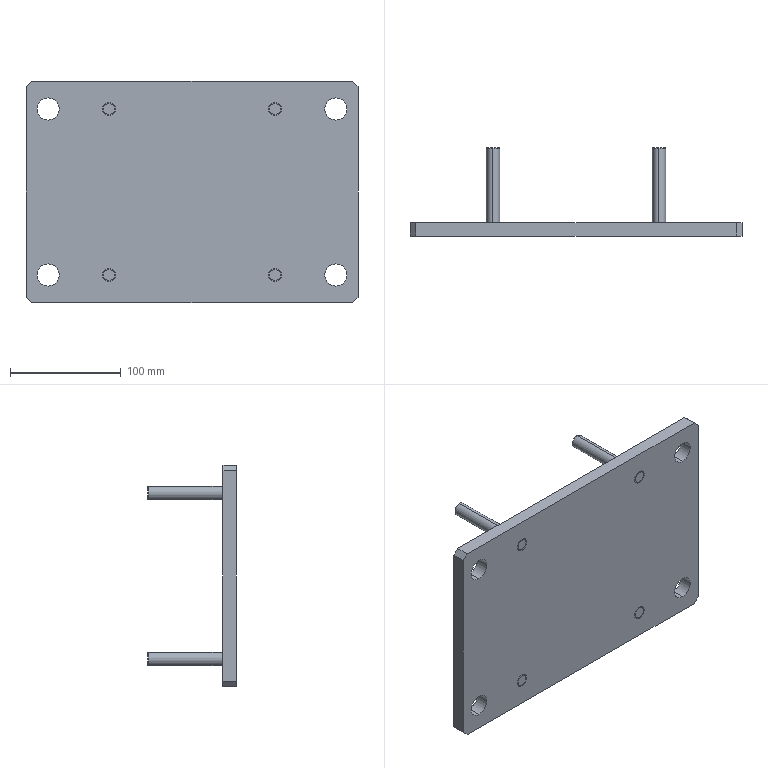Part | SolidWorks | features Chamfer 2, HoleWzd 2, Extrusion 1, ICE 1, SketchPattern 1 | 6 solids | 56 faces | box 300 x 80 x 200 mm | volume 745614 mm3 | cylinder 26 | plane 20 | cone 10 | commonest cylinder face diameters 12 x10 10.2 x8 20 x8
STEP:
#1=CARTESIAN_POINT('',(75.,74.,80.5));
#2=VERTEX_POINT('',#1);
#3=CARTESIAN_POINT('',(75.,74.,69.5));
#4=VERTEX_POINT('',#3);
#5=CARTESIAN_POINT('',(75.,74.,75.));
#6=DIRECTION('',(0.,1.,0.));
#7=DIRECTION('',(0.,0.,-1.));
#8=AXIS2_PLACEMENT_3D('',#5,#6,#7);
#9=CIRCLE('',#8,5.5);
#10=EDGE_CURVE('',#2,#4,#9,.T.);
#11=ORIENTED_EDGE('',*,*,#10,.F.);
#12=CARTESIAN_POINT('',(75.,73.5,81.));
#13=VERTEX_POINT('',#12);
#14=CARTESIAN_POINT('',(75.,73.5,81.));
#15=DIRECTION('',(0.,-0.7071,0.7071));
#16=VECTOR('',#15,1000.);
#17=LINE('',#14,#16);
#18=EDGE_CURVE('',#2,#13,#17,.T.);
#19=ORIENTED_EDGE('',*,*,#18,.T.);
#20=CARTESIAN_POINT('',(75.,73.5,69.));
#21=VERTEX_POINT('',#20);
#22=CARTESIAN_POINT('',(75.,73.5,75.));
#23=DIRECTION('',(0.,-1.,0.));
#24=DIRECTION('',(0.,0.,-1.));
#25=AXIS2_PLACEMENT_3D('',#22,#23,#24);
#26=CIRCLE('',#25,6.);
#27=EDGE_CURVE('',#21,#13,#26,.T.);
#28=ORIENTED_EDGE('',*,*,#27,.F.);
#29=CARTESIAN_POINT('',(75.,73.5,69.));
#30=DIRECTION('',(0.,-0.7071,-0.7071));
#31=VECTOR('',#30,1000.);
#32=LINE('',#29,#31);
#33=EDGE_CURVE('',#4,#21,#32,.T.);
#34=ORIENTED_EDGE('',*,*,#33,.F.);
#35=EDGE_LOOP('',(#11,#19,#28,#34));
#36=FACE_OUTER_BOUND('',#35,.T.);
#37=CARTESIAN_POINT('',(75.,73.5,75.));
#38=DIRECTION('',(0.,-1.,0.));
#39=DIRECTION('',(0.,0.,-1.));
#40=AXIS2_PLACEMENT_3D('',#37,#38,#39);
#41=CONICAL_SURFACE('',#40,6.,0.7854);
#42=ADVANCED_FACE('',(#36),#41,.T.);
#43=ORIENTED_EDGE('',*,*,#27,.T.);
#44=CARTESIAN_POINT('',(75.,-6.,81.));
#45=VERTEX_POINT('',#44);
#46=CARTESIAN_POINT('',(75.,74.,81.));
#47=DIRECTION('',(0.,-1.,0.));
#48=VECTOR('',#47,1000.);
#49=LINE('',#46,#48);
#50=EDGE_CURVE('',#13,#45,#49,.T.);
#51=ORIENTED_EDGE('',*,*,#50,.T.);
#52=CARTESIAN_POINT('',(75.,-6.,69.));
#53=VERTEX_POINT('',#52);
#54=CARTESIAN_POINT('',(75.,-6.,75.));
#55=DIRECTION('',(0.,-1.,0.));
#56=DIRECTION('',(0.,0.,-1.));
#57=AXIS2_PLACEMENT_3D('',#54,#55,#56);
#58=CIRCLE('',#57,6.);
#59=EDGE_CURVE('',#53,#45,#58,.T.);
#60=ORIENTED_EDGE('',*,*,#59,.F.);
#61=CARTESIAN_POINT('',(75.,74.,69.));
#62=DIRECTION('',(0.,-1.,0.));
#63=VECTOR('',#62,1000.);
#64=LINE('',#61,#63);
#65=EDGE_CURVE('',#21,#53,#64,.T.);
#66=ORIENTED_EDGE('',*,*,#65,.F.);
#67=EDGE_LOOP('',(#43,#51,#60,#66));
#68=FACE_OUTER_BOUND('',#67,.T.);
#69=CARTESIAN_POINT('',(75.,74.,75.));
#70=DIRECTION('',(0.,-1.,0.));
#71=DIRECTION('',(0.,0.,-1.));
#72=AXIS2_PLACEMENT_3D('',#69,#70,#71);
#73=CYLINDRICAL_SURFACE('',#72,6.);
#74=ADVANCED_FACE('',(#68),#73,.T.);
#75=ORIENTED_EDGE('',*,*,#50,.F.);
#76=CARTESIAN_POINT('',(75.,73.5,75.));
#77=DIRECTION('',(0.,-1.,0.));
#78=DIRECTION('',(0.,0.,-1.));
#79=AXIS2_PLACEMENT_3D('',#76,#77,#78);
#80=CIRCLE('',#79,6.);
#81=EDGE_CURVE('',#13,#21,#80,.T.);
#82=ORIENTED_EDGE('',*,*,#81,.T.);
#83=ORIENTED_EDGE('',*,*,#65,.T.);
#84=CARTESIAN_POINT('',(75.,-6.,75.));
#85=DIRECTION('',(0.,-1.,0.));
#86=DIRECTION('',(0.,0.,-1.));
#87=AXIS2_PLACEMENT_3D('',#84,#85,#86);
#88=CIRCLE('',#87,6.);
#89=EDGE_CURVE('',#45,#53,#88,.T.);
#90=ORIENTED_EDGE('',*,*,#89,.F.);
#91=EDGE_LOOP('',(#75,#82,#83,#90));
#92=FACE_OUTER_BOUND('',#91,.T.);
#93=CARTESIAN_POINT('',(75.,74.,75.));
#94=DIRECTION('',(0.,-1.,0.));
#95=DIRECTION('',(0.,0.,-1.));
#96=AXIS2_PLACEMENT_3D('',#93,#94,#95);
#97=CYLINDRICAL_SURFACE('',#96,6.);
#98=ADVANCED_FACE('',(#92),#97,.T.);
#99=CARTESIAN_POINT('',(75.,74.,75.));
#100=DIRECTION('',(0.,1.,0.));
#101=DIRECTION('',(0.,0.,-1.));
#102=AXIS2_PLACEMENT_3D('',#99,#100,#101);
#103=CIRCLE('',#102,5.5);
#104=EDGE_CURVE('',#4,#2,#103,.T.);
#105=ORIENTED_EDGE('',*,*,#104,.T.);
#106=ORIENTED_EDGE('',*,*,#10,.T.);
#107=EDGE_LOOP('',(#105,#106));
#108=FACE_OUTER_BOUND('',#107,.T.);
#109=CARTESIAN_POINT('',(75.,74.,75.));
#110=DIRECTION('',(0.,-1.,0.));
#111=DIRECTION('',(0.,0.,-1.));
#112=AXIS2_PLACEMENT_3D('',#109,#110,#111);
#113=PLANE('',#112);
#114=ADVANCED_FACE('',(#108),#113,.F.);
#115=ORIENTED_EDGE('',*,*,#59,.T.);
#116=ORIENTED_EDGE('',*,*,#89,.T.);
#117=EDGE_LOOP('',(#115,#116));
#118=FACE_OUTER_BOUND('',#117,.T.);
#119=CARTESIAN_POINT('',(75.,-6.,75.));
#120=DIRECTION('',(0.,-1.,0.));
#121=DIRECTION('',(0.,0.,-1.));
#122=AXIS2_PLACEMENT_3D('',#119,#120,#121);
#123=PLANE('',#122);
#124=ADVANCED_FACE('',(#118),#123,.T.);
#125=ORIENTED_EDGE('',*,*,#18,.F.);
#126=ORIENTED_EDGE('',*,*,#104,.F.);
#127=ORIENTED_EDGE('',*,*,#33,.T.);
#128=ORIENTED_EDGE('',*,*,#81,.F.);
#129=EDGE_LOOP('',(#125,#126,#127,#128));
#130=FACE_OUTER_BOUND('',#129,.T.);
#131=CARTESIAN_POINT('',(75.,73.5,75.));
#132=DIRECTION('',(0.,-1.,0.));
#133=DIRECTION('',(0.,0.,-1.));
#134=AXIS2_PLACEMENT_3D('',#131,#132,#133);
#135=CONICAL_SURFACE('',#134,6.,0.7854);
#136=ADVANCED_FACE('',(#130),#135,.T.);
#137=CLOSED_SHELL('',(#42,#74,#98,#114,#124,#136));
#138=MANIFOLD_SOLID_BREP('',#137);
#139=CARTESIAN_POINT('',(75.,74.,80.5));
#140=VERTEX_POINT('',#139);
#141=CARTESIAN_POINT('',(75.,74.,69.5));
#142=VERTEX_POINT('',#141);
#143=CARTESIAN_POINT('',(75.,74.,75.));
#144=DIRECTION('',(0.,1.,0.));
#145=DIRECTION('',(0.,0.,-1.));
#146=AXIS2_PLACEMENT_3D('',#143,#144,#145);
#147=CIRCLE('',#146,5.5);
#148=EDGE_CURVE('',#140,#142,#147,.T.);
#149=ORIENTED_EDGE('',*,*,#148,.F.);
#150=CARTESIAN_POINT('',(75.,73.5,81.));
#151=VERTEX_POINT('',#150);
#152=CARTESIAN_POINT('',(75.,73.5,81.));
#153=DIRECTION('',(0.,-0.7071,0.7071));
#154=VECTOR('',#153,1000.);
#155=LINE('',#152,#154);
#156=EDGE_CURVE('',#140,#151,#155,.T.);
#157=ORIENTED_EDGE('',*,*,#156,.T.);
#158=CARTESIAN_POINT('',(75.,73.5,69.));
#159=VERTEX_POINT('',#158);
#160=CARTESIAN_POINT('',(75.,73.5,75.));
#161=DIRECTION('',(0.,-1.,0.));
#162=DIRECTION('',(0.,0.,-1.));
#163=AXIS2_PLACEMENT_3D('',#160,#161,#162);
#164=CIRCLE('',#163,6.);
#165=EDGE_CURVE('',#159,#151,#164,.T.);
#166=ORIENTED_EDGE('',*,*,#165,.F.);
#167=CARTESIAN_POINT('',(75.,73.5,69.));
#168=DIRECTION('',(0.,-0.7071,-0.7071));
#169=VECTOR('',#168,1000.);
#170=LINE('',#167,#169);
#171=EDGE_CURVE('',#142,#159,#170,.T.);
#172=ORIENTED_EDGE('',*,*,#171,.F.);
#173=EDGE_LOOP('',(#149,#157,#166,#172));
#174=FACE_OUTER_BOUND('',#173,.T.);
#175=CARTESIAN_POINT('',(75.,73.5,75.));
#176=DIRECTION('',(0.,-1.,0.));
#177=DIRECTION('',(0.,0.,-1.));
#178=AXIS2_PLACEMENT_3D('',#175,#176,#177);
#179=CONICAL_SURFACE('',#178,6.,0.7854);
#180=ADVANCED_FACE('',(#174),#179,.T.);
#181=ORIENTED_EDGE('',*,*,#165,.T.);
#182=CARTESIAN_POINT('',(75.,-6.,81.));
#183=VERTEX_POINT('',#182);
#184=CARTESIAN_POINT('',(75.,74.,81.));
#185=DIRECTION('',(0.,-1.,0.));
#186=VECTOR('',#185,1000.);
#187=LINE('',#184,#186);
#188=EDGE_CURVE('',#151,#183,#187,.T.);
#189=ORIENTED_EDGE('',*,*,#188,.T.);
#190=CARTESIAN_POINT('',(75.,-6.,69.));
#191=VERTEX_POINT('',#190);
#192=CARTESIAN_POINT('',(75.,-6.,75.));
#193=DIRECTION('',(0.,-1.,0.));
#194=DIRECTION('',(0.,0.,-1.));
#195=AXIS2_PLACEMENT_3D('',#192,#193,#194);
#196=CIRCLE('',#195,6.);
#197=EDGE_CURVE('',#191,#183,#196,.T.);
#198=ORIENTED_EDGE('',*,*,#197,.F.);
#199=CARTESIAN_POINT('',(75.,74.,69.));
#200=DIRECTION('',(0.,-1.,0.));
#201=VECTOR('',#200,1000.);
#202=LINE('',#199,#201);
#203=EDGE_CURVE('',#159,#191,#202,.T.);
#204=ORIENTED_EDGE('',*,*,#203,.F.);
#205=EDGE_LOOP('',(#181,#189,#198,#204));
#206=FACE_OUTER_BOUND('',#205,.T.);
#207=CARTESIAN_POINT('',(75.,74.,75.));
#208=DIRECTION('',(0.,-1.,0.));
#209=DIRECTION('',(0.,0.,-1.));
#210=AXIS2_PLACEMENT_3D('',#207,#208,#209);
#211=CYLINDRICAL_SURFACE('',#210,6.);
#212=ADVANCED_FACE('',(#206),#211,.T.);
#213=ORIENTED_EDGE('',*,*,#188,.F.);
#214=CARTESIAN_POINT('',(75.,73.5,75.));
#215=DIRECTION('',(0.,-1.,0.));
#216=DIRECTION('',(0.,0.,-1.));
#217=AXIS2_PLACEMENT_3D('',#214,#215,#216);
#218=CIRCLE('',#217,6.);
#219=EDGE_CURVE('',#151,#159,#218,.T.);
#220=ORIENTED_EDGE('',*,*,#219,.T.);
#221=ORIENTED_EDGE('',*,*,#203,.T.);
#222=CARTESIAN_POINT('',(75.,-6.,75.));
#223=DIRECTION('',(0.,-1.,0.));
#224=DIRECTION('',(0.,0.,-1.));
#225=AXIS2_PLACEMENT_3D('',#222,#223,#224);
#226=CIRCLE('',#225,6.);
#227=EDGE_CURVE('',#183,#191,#226,.T.);
#228=ORIENTED_EDGE('',*,*,#227,.F.);
#229=EDGE_LOOP('',(#213,#220,#221,#228));
#230=FACE_OUTER_BOUND('',#229,.T.);
#231=CARTESIAN_POINT('',(75.,74.,75.));
#232=DIRECTION('',(0.,-1.,0.));
#233=DIRECTION('',(0.,0.,-1.));
#234=AXIS2_PLACEMENT_3D('',#231,#232,#233);
#235=CYLINDRICAL_SURFACE('',#234,6.);
#236=ADVANCED_FACE('',(#230),#235,.T.);
#237=CARTESIAN_POINT('',(75.,74.,75.));
#238=DIRECTION('',(0.,1.,0.));
#239=DIRECTION('',(0.,0.,-1.));
#240=AXIS2_PLACEMENT_3D('',#237,#238,#239);
#241=CIRCLE('',#240,5.5);
#242=EDGE_CURVE('',#142,#140,#241,.T.);
#243=ORIENTED_EDGE('',*,*,#242,.T.);
#244=ORIENTED_EDGE('',*,*,#148,.T.);
#245=EDGE_LOOP('',(#243,#244));
#246=FACE_OUTER_BOUND('',#245,.T.);
#247=CARTESIAN_POINT('',(75.,74.,75.));
#248=DIRECTION('',(0.,-1.,0.));
#249=DIRECTION('',(0.,0.,-1.));
#250=AXIS2_PLACEMENT_3D('',#247,#248,#249);
#251=PLANE('',#250);
#252=ADVANCED_FACE('',(#246),#251,.F.);
#253=ORIENTED_EDGE('',*,*,#197,.T.);
#254=ORIENTED_EDGE('',*,*,#227,.T.);
#255=EDGE_LOOP('',(#253,#254));
#256=FACE_OUTER_BOUND('',#255,.T.);
#257=CARTESIAN_POINT('',(75.,-6.,75.));
#258=DIRECTION('',(0.,-1.,0.));
#259=DIRECTION('',(0.,0.,-1.));
#260=AXIS2_PLACEMENT_3D('',#257,#258,#259);
#261=PLANE('',#260);
#262=ADVANCED_FACE('',(#256),#261,.T.);
#263=ORIENTED_EDGE('',*,*,#156,.F.);
#264=ORIENTED_EDGE('',*,*,#242,.F.);
#265=ORIENTED_EDGE('',*,*,#171,.T.);
#266=ORIENTED_EDGE('',*,*,#219,.F.);
#267=EDGE_LOOP('',(#263,#264,#265,#266));
#268=FACE_OUTER_BOUND('',#267,.T.);
#269=CARTESIAN_POINT('',(75.,73.5,75.));
#270=DIRECTION('',(0.,-1.,0.));
#271=DIRECTION('',(0.,0.,-1.));
#272=AXIS2_PLACEMENT_3D('',#269,#270,#271);
#273=CONICAL_SURFACE('',#272,6.,0.7854);
#274=ADVANCED_FACE('',(#268),#273,.T.);
#275=CLOSED_SHELL('',(#180,#212,#236,#252,#262,#274));
#276=MANIFOLD_SOLID_BREP('',#275);
#277=CARTESIAN_POINT('',(75.,74.,-69.5));
#278=VERTEX_POINT('',#277);
#279=CARTESIAN_POINT('',(75.,74.,-80.5));
#280=VERTEX_POINT('',#279);
#281=CARTESIAN_POINT('',(75.,74.,-75.));
#282=DIRECTION('',(0.,1.,0.));
#283=DIRECTION('',(0.,0.,-1.));
#284=AXIS2_PLACEMENT_3D('',#281,#282,#283);
#285=CIRCLE('',#284,5.5);
#286=EDGE_CURVE('',#278,#280,#285,.T.);
#287=ORIENTED_EDGE('',*,*,#286,.F.);
#288=CARTESIAN_POINT('',(75.,73.5,-69.));
#289=VERTEX_POINT('',#288);
#290=CARTESIAN_POINT('',(75.,73.5,-69.));
#291=DIRECTION('',(0.,-0.7071,0.7071));
#292=VECTOR('',#291,1000.);
#293=LINE('',#290,#292);
#294=EDGE_CURVE('',#278,#289,#293,.T.);
#295=ORIENTED_EDGE('',*,*,#294,.T.);
#296=CARTESIAN_POINT('',(75.,73.5,-81.));
#297=VERTEX_POINT('',#296);
#298=CARTESIAN_POINT('',(75.,73.5,-75.));
#299=DIRECTION('',(0.,-1.,0.));
#300=DIRECTION('',(0.,0.,-1.));
#301=AXIS2_PLACEMENT_3D('',#298,#299,#300);
#302=CIRCLE('',#301,6.);
#303=EDGE_CURVE('',#297,#289,#302,.T.);
#304=ORIENTED_EDGE('',*,*,#303,.F.);
#305=CARTESIAN_POINT('',(75.,73.5,-81.));
#306=DIRECTION('',(0.,-0.7071,-0.7071));
#307=VECTOR('',#306,1000.);
#308=LINE('',#305,#307);
#309=EDGE_CURVE('',#280,#297,#308,.T.);
#310=ORIENTED_EDGE('',*,*,#309,.F.);
#311=EDGE_LOOP('',(#287,#295,#304,#310));
#312=FACE_OUTER_BOUND('',#311,.T.);
#313=CARTESIAN_POINT('',(75.,73.5,-75.));
#314=DIRECTION('',(0.,-1.,0.));
#315=DIRECTION('',(0.,0.,-1.));
#316=AXIS2_PLACEMENT_3D('',#313,#314,#315);
#317=CONICAL_SURFACE('',#316,6.,0.7854);
#318=ADVANCED_FACE('',(#312),#317,.T.);
#319=ORIENTED_EDGE('',*,*,#303,.T.);
#320=CARTESIAN_POINT('',(75.,-6.,-69.));
#321=VERTEX_POINT('',#320);
#322=CARTESIAN_POINT('',(75.,74.,-69.));
#323=DIRECTION('',(0.,-1.,0.));
#324=VECTOR('',#323,1000.);
#325=LINE('',#322,#324);
#326=EDGE_CURVE('',#289,#321,#325,.T.);
#327=ORIENTED_EDGE('',*,*,#326,.T.);
#328=CARTESIAN_POINT('',(75.,-6.,-81.));
#329=VERTEX_POINT('',#328);
#330=CARTESIAN_POINT('',(75.,-6.,-75.));
#331=DIRECTION('',(0.,-1.,0.));
#332=DIRECTION('',(0.,0.,-1.));
#333=AXIS2_PLACEMENT_3D('',#330,#331,#332);
#334=CIRCLE('',#333,6.);
#335=EDGE_CURVE('',#329,#321,#334,.T.);
#336=ORIENTED_EDGE('',*,*,#335,.F.);
#337=CARTESIAN_POINT('',(75.,74.,-81.));
#338=DIRECTION('',(0.,-1.,0.));
#339=VECTOR('',#338,1000.);
#340=LINE('',#337,#339);
#341=EDGE_CURVE('',#297,#329,#340,.T.);
#342=ORIENTED_EDGE('',*,*,#341,.F.);
#343=EDGE_LOOP('',(#319,#327,#336,#342));
#344=FACE_OUTER_BOUND('',#343,.T.);
#345=CARTESIAN_POINT('',(75.,74.,-75.));
#346=DIRECTION('',(0.,-1.,0.));
#347=DIRECTION('',(0.,0.,-1.));
#348=AXIS2_PLACEMENT_3D('',#345,#346,#347);
#349=CYLINDRICAL_SURFACE('',#348,6.);
#350=ADVANCED_FACE('',(#344),#349,.T.);
#351=ORIENTED_EDGE('',*,*,#326,.F.);
#352=CARTESIAN_POINT('',(75.,73.5,-75.));
#353=DIRECTION('',(0.,-1.,0.));
#354=DIRECTION('',(0.,0.,-1.));
#355=AXIS2_PLACEMENT_3D('',#352,#353,#354);
#356=CIRCLE('',#355,6.);
#357=EDGE_CURVE('',#289,#297,#356,.T.);
#358=ORIENTED_EDGE('',*,*,#357,.T.);
#359=ORIENTED_EDGE('',*,*,#341,.T.);
#360=CARTESIAN_POINT('',(75.,-6.,-75.));
#361=DIRECTION('',(0.,-1.,0.));
#362=DIRECTION('',(0.,0.,-1.));
#363=AXIS2_PLACEMENT_3D('',#360,#361,#362);
#364=CIRCLE('',#363,6.);
#365=EDGE_CURVE('',#321,#329,#364,.T.);
#366=ORIENTED_EDGE('',*,*,#365,.F.);
#367=EDGE_LOOP('',(#351,#358,#359,#366));
#368=FACE_OUTER_BOUND('',#367,.T.);
#369=CARTESIAN_POINT('',(75.,74.,-75.));
#370=DIRECTION('',(0.,-1.,0.));
#371=DIRECTION('',(0.,0.,-1.));
#372=AXIS2_PLACEMENT_3D('',#369,#370,#371);
#373=CYLINDRICAL_SURFACE('',#372,6.);
#374=ADVANCED_FACE('',(#368),#373,.T.);
#375=CARTESIAN_POINT('',(75.,74.,-75.));
#376=DIRECTION('',(0.,1.,0.));
#377=DIRECTION('',(0.,0.,-1.));
#378=AXIS2_PLACEMENT_3D('',#375,#376,#377);
#379=CIRCLE('',#378,5.5);
#380=EDGE_CURVE('',#280,#278,#379,.T.);
#381=ORIENTED_EDGE('',*,*,#380,.T.);
#382=ORIENTED_EDGE('',*,*,#286,.T.);
#383=EDGE_LOOP('',(#381,#382));
#384=FACE_OUTER_BOUND('',#383,.T.);
#385=CARTESIAN_POINT('',(75.,74.,-75.));
#386=DIRECTION('',(0.,-1.,0.));
#387=DIRECTION('',(0.,0.,-1.));
#388=AXIS2_PLACEMENT_3D('',#385,#386,#387);
#389=PLANE('',#388);
#390=ADVANCED_FACE('',(#384),#389,.F.);
#391=ORIENTED_EDGE('',*,*,#335,.T.);
#392=ORIENTED_EDGE('',*,*,#365,.T.);
#393=EDGE_LOOP('',(#391,#392));
#394=FACE_OUTER_BOUND('',#393,.T.);
#395=CARTESIAN_POINT('',(75.,-6.,-75.));
#396=DIRECTION('',(0.,-1.,0.));
#397=DIRECTION('',(0.,0.,-1.));
#398=AXIS2_PLACEMENT_3D('',#395,#396,#397);
#399=PLANE('',#398);
#400=ADVANCED_FACE('',(#394),#399,.T.);
#401=ORIENTED_EDGE('',*,*,#294,.F.);
#402=ORIENTED_EDGE('',*,*,#380,.F.);
#403=ORIENTED_EDGE('',*,*,#309,.T.);
#404=ORIENTED_EDGE('',*,*,#357,.F.);
#405=EDGE_LOOP('',(#401,#402,#403,#404));
#406=FACE_OUTER_BOUND('',#405,.T.);
#407=CARTESIAN_POINT('',(75.,73.5,-75.));
#408=DIRECTION('',(0.,-1.,0.));
#409=DIRECTION('',(0.,0.,-1.));
#410=AXIS2_PLACEMENT_3D('',#407,#408,#409);
#411=CONICAL_SURFACE('',#410,6.,0.7854);
#412=ADVANCED_FACE('',(#406),#411,.T.);
#413=CLOSED_SHELL('',(#318,#350,#374,#390,#400,#412));
#414=MANIFOLD_SOLID_BREP('',#413);
#415=CARTESIAN_POINT('',(-75.,74.,-69.5));
#416=VERTEX_POINT('',#415);
#417=CARTESIAN_POINT('',(-75.,74.,-80.5));
#418=VERTEX_POINT('',#417);
#419=CARTESIAN_POINT('',(-75.,74.,-75.));
#420=DIRECTION('',(0.,1.,0.));
#421=DIRECTION('',(0.,0.,-1.));
#422=AXIS2_PLACEMENT_3D('',#419,#420,#421);
#423=CIRCLE('',#422,5.5);
#424=EDGE_CURVE('',#416,#418,#423,.T.);
#425=ORIENTED_EDGE('',*,*,#424,.F.);
#426=CARTESIAN_POINT('',(-75.,73.5,-69.));
#427=VERTEX_POINT('',#426);
#428=CARTESIAN_POINT('',(-75.,73.5,-69.));
#429=DIRECTION('',(0.,-0.7071,0.7071));
#430=VECTOR('',#429,1000.);
#431=LINE('',#428,#430);
#432=EDGE_CURVE('',#416,#427,#431,.T.);
#433=ORIENTED_EDGE('',*,*,#432,.T.);
#434=CARTESIAN_POINT('',(-75.,73.5,-81.));
#435=VERTEX_POINT('',#434);
#436=CARTESIAN_POINT('',(-75.,73.5,-75.));
#437=DIRECTION('',(0.,-1.,0.));
#438=DIRECTION('',(0.,0.,-1.));
#439=AXIS2_PLACEMENT_3D('',#436,#437,#438);
#440=CIRCLE('',#439,6.);
#441=EDGE_CURVE('',#435,#427,#440,.T.);
#442=ORIENTED_EDGE('',*,*,#441,.F.);
#443=CARTESIAN_POINT('',(-75.,73.5,-81.));
#444=DIRECTION('',(0.,-0.7071,-0.7071));
#445=VECTOR('',#444,1000.);
#446=LINE('',#443,#445);
#447=EDGE_CURVE('',#418,#435,#446,.T.);
#448=ORIENTED_EDGE('',*,*,#447,.F.);
#449=EDGE_LOOP('',(#425,#433,#442,#448));
#450=FACE_OUTER_BOUND('',#449,.T.);
#451=CARTESIAN_POINT('',(-75.,73.5,-75.));
#452=DIRECTION('',(0.,-1.,0.));
#453=DIRECTION('',(0.,0.,-1.));
#454=AXIS2_PLACEMENT_3D('',#451,#452,#453);
#455=CONICAL_SURFACE('',#454,6.,0.7854);
#456=ADVANCED_FACE('',(#450),#455,.T.);
#457=ORIENTED_EDGE('',*,*,#441,.T.);
#458=CARTESIAN_POINT('',(-75.,-6.,-69.));
#459=VERTEX_POINT('',#458);
#460=CARTESIAN_POINT('',(-75.,74.,-69.));
#461=DIRECTION('',(0.,-1.,0.));
#462=VECTOR('',#461,1000.);
#463=LINE('',#460,#462);
#464=EDGE_CURVE('',#427,#459,#463,.T.);
#465=ORIENTED_EDGE('',*,*,#464,.T.);
#466=CARTESIAN_POINT('',(-75.,-6.,-81.));
#467=VERTEX_POINT('',#466);
#468=CARTESIAN_POINT('',(-75.,-6.,-75.));
#469=DIRECTION('',(0.,-1.,0.));
#470=DIRECTION('',(0.,0.,-1.));
#471=AXIS2_PLACEMENT_3D('',#468,#469,#470);
#472=CIRCLE('',#471,6.);
#473=EDGE_CURVE('',#467,#459,#472,.T.);
#474=ORIENTED_EDGE('',*,*,#473,.F.);
#475=CARTESIAN_POINT('',(-75.,74.,-81.));
#476=DIRECTION('',(0.,-1.,0.));
#477=VECTOR('',#476,1000.);
#478=LINE('',#475,#477);
#479=EDGE_CURVE('',#435,#467,#478,.T.);
#480=ORIENTED_EDGE('',*,*,#479,.F.);
#481=EDGE_LOOP('',(#457,#465,#474,#480));
#482=FACE_OUTER_BOUND('',#481,.T.);
#483=CARTESIAN_POINT('',(-75.,74.,-75.));
#484=DIRECTION('',(0.,-1.,0.));
#485=DIRECTION('',(0.,0.,-1.));
#486=AXIS2_PLACEMENT_3D('',#483,#484,#485);
#487=CYLINDRICAL_SURFACE('',#486,6.);
#488=ADVANCED_FACE('',(#482),#487,.T.);
#489=ORIENTED_EDGE('',*,*,#464,.F.);
#490=CARTESIAN_POINT('',(-75.,73.5,-75.));
#491=DIRECTION('',(0.,-1.,0.));
#492=DIRECTION('',(0.,0.,-1.));
#493=AXIS2_PLACEMENT_3D('',#490,#491,#492);
#494=CIRCLE('',#493,6.);
#495=EDGE_CURVE('',#427,#435,#494,.T.);
#496=ORIENTED_EDGE('',*,*,#495,.T.);
#497=ORIENTED_EDGE('',*,*,#479,.T.);
#498=CARTESIAN_POINT('',(-75.,-6.,-75.));
#499=DIRECTION('',(0.,-1.,0.));
#500=DIRECTION('',(0.,0.,-1.));
#501=AXIS2_PLACEMENT_3D('',#498,#499,#500);
#502=CIRCLE('',#501,6.);
#503=EDGE_CURVE('',#459,#467,#502,.T.);
#504=ORIENTED_EDGE('',*,*,#503,.F.);
#505=EDGE_LOOP('',(#489,#496,#497,#504));
#506=FACE_OUTER_BOUND('',#505,.T.);
#507=CARTESIAN_POINT('',(-75.,74.,-75.));
#508=DIRECTION('',(0.,-1.,0.));
#509=DIRECTION('',(0.,0.,-1.));
#510=AXIS2_PLACEMENT_3D('',#507,#508,#509);
#511=CYLINDRICAL_SURFACE('',#510,6.);
#512=ADVANCED_FACE('',(#506),#511,.T.);
#513=CARTESIAN_POINT('',(-75.,74.,-75.));
#514=DIRECTION('',(0.,1.,0.));
#515=DIRECTION('',(0.,0.,-1.));
#516=AXIS2_PLACEMENT_3D('',#513,#514,#515);
#517=CIRCLE('',#516,5.5);
#518=EDGE_CURVE('',#418,#416,#517,.T.);
#519=ORIENTED_EDGE('',*,*,#518,.T.);
#520=ORIENTED_EDGE('',*,*,#424,.T.);
#521=EDGE_LOOP('',(#519,#520));
#522=FACE_OUTER_BOUND('',#521,.T.);
#523=CARTESIAN_POINT('',(-75.,74.,-75.));
#524=DIRECTION('',(0.,-1.,0.));
#525=DIRECTION('',(0.,0.,-1.));
#526=AXIS2_PLACEMENT_3D('',#523,#524,#525);
#527=PLANE('',#526);
#528=ADVANCED_FACE('',(#522),#527,.F.);
#529=ORIENTED_EDGE('',*,*,#473,.T.);
#530=ORIENTED_EDGE('',*,*,#503,.T.);
#531=EDGE_LOOP('',(#529,#530));
#532=FACE_OUTER_BOUND('',#531,.T.);
#533=CARTESIAN_POINT('',(-75.,-6.,-75.));
#534=DIRECTION('',(0.,-1.,0.));
#535=DIRECTION('',(0.,0.,-1.));
#536=AXIS2_PLACEMENT_3D('',#533,#534,#535);
#537=PLANE('',#536);
#538=ADVANCED_FACE('',(#532),#537,.T.);
#539=ORIENTED_EDGE('',*,*,#432,.F.);
#540=ORIENTED_EDGE('',*,*,#518,.F.);
#541=ORIENTED_EDGE('',*,*,#447,.T.);
#542=ORIENTED_EDGE('',*,*,#495,.F.);
#543=EDGE_LOOP('',(#539,#540,#541,#542));
#544=FACE_OUTER_BOUND('',#543,.T.);
#545=CARTESIAN_POINT('',(-75.,73.5,-75.));
#546=DIRECTION('',(0.,-1.,0.));
#547=DIRECTION('',(0.,0.,-1.));
#548=AXIS2_PLACEMENT_3D('',#545,#546,#547);
#549=CONICAL_SURFACE('',#548,6.,0.7854);
#550=ADVANCED_FACE('',(#544),#549,.T.);
#551=CLOSED_SHELL('',(#456,#488,#512,#528,#538,#550));
#552=MANIFOLD_SOLID_BREP('',#551);
#553=CARTESIAN_POINT('',(-75.,74.,80.5));
#554=VERTEX_POINT('',#553);
#555=CARTESIAN_POINT('',(-75.,74.,69.5));
#556=VERTEX_POINT('',#555);
#557=CARTESIAN_POINT('',(-75.,74.,75.));
#558=DIRECTION('',(0.,1.,0.));
#559=DIRECTION('',(0.,0.,-1.));
#560=AXIS2_PLACEMENT_3D('',#557,#558,#559);
#561=CIRCLE('',#560,5.5);
#562=EDGE_CURVE('',#554,#556,#561,.T.);
#563=ORIENTED_EDGE('',*,*,#562,.F.);
#564=CARTESIAN_POINT('',(-75.,73.5,81.));
#565=VERTEX_POINT('',#564);
#566=CARTESIAN_POINT('',(-75.,73.5,81.));
#567=DIRECTION('',(0.,-0.7071,0.7071));
#568=VECTOR('',#567,1000.);
#569=LINE('',#566,#568);
#570=EDGE_CURVE('',#554,#565,#569,.T.);
#571=ORIENTED_EDGE('',*,*,#570,.T.);
#572=CARTESIAN_POINT('',(-75.,73.5,69.));
#573=VERTEX_POINT('',#572);
#574=CARTESIAN_POINT('',(-75.,73.5,75.));
#575=DIRECTION('',(0.,-1.,0.));
#576=DIRECTION('',(0.,0.,-1.));
#577=AXIS2_PLACEMENT_3D('',#574,#575,#576);
#578=CIRCLE('',#577,6.);
#579=EDGE_CURVE('',#573,#565,#578,.T.);
#580=ORIENTED_EDGE('',*,*,#579,.F.);
#581=CARTESIAN_POINT('',(-75.,73.5,69.));
#582=DIRECTION('',(0.,-0.7071,-0.7071));
#583=VECTOR('',#582,1000.);
#584=LINE('',#581,#583);
#585=EDGE_CURVE('',#556,#573,#584,.T.);
#586=ORIENTED_EDGE('',*,*,#585,.F.);
#587=EDGE_LOOP('',(#563,#571,#580,#586));
#588=FACE_OUTER_BOUND('',#587,.T.);
#589=CARTESIAN_POINT('',(-75.,73.5,75.));
#590=DIRECTION('',(0.,-1.,0.));
#591=DIRECTION('',(0.,0.,-1.));
#592=AXIS2_PLACEMENT_3D('',#589,#590,#591);
#593=CONICAL_SURFACE('',#592,6.,0.7854);
#594=ADVANCED_FACE('',(#588),#593,.T.);
#595=ORIENTED_EDGE('',*,*,#579,.T.);
#596=CARTESIAN_POINT('',(-75.,-6.,81.));
#597=VERTEX_POINT('',#596);
#598=CARTESIAN_POINT('',(-75.,74.,81.));
#599=DIRECTION('',(0.,-1.,0.));
#600=VECTOR('',#599,1000.);
#601=LINE('',#598,#600);
#602=EDGE_CURVE('',#565,#597,#601,.T.);
#603=ORIENTED_EDGE('',*,*,#602,.T.);
#604=CARTESIAN_POINT('',(-75.,-6.,69.));
#605=VERTEX_POINT('',#604);
#606=CARTESIAN_POINT('',(-75.,-6.,75.));
#607=DIRECTION('',(0.,-1.,0.));
#608=DIRECTION('',(0.,0.,-1.));
#609=AXIS2_PLACEMENT_3D('',#606,#607,#608);
#610=CIRCLE('',#609,6.);
#611=EDGE_CURVE('',#605,#597,#610,.T.);
#612=ORIENTED_EDGE('',*,*,#611,.F.);
#613=CARTESIAN_POINT('',(-75.,74.,69.));
#614=DIRECTION('',(0.,-1.,0.));
#615=VECTOR('',#614,1000.);
#616=LINE('',#613,#615);
#617=EDGE_CURVE('',#573,#605,#616,.T.);
#618=ORIENTED_EDGE('',*,*,#617,.F.);
#619=EDGE_LOOP('',(#595,#603,#612,#618));
#620=FACE_OUTER_BOUND('',#619,.T.);
#621=CARTESIAN_POINT('',(-75.,74.,75.));
#622=DIRECTION('',(0.,-1.,0.));
#623=DIRECTION('',(0.,0.,-1.));
#624=AXIS2_PLACEMENT_3D('',#621,#622,#623);
#625=CYLINDRICAL_SURFACE('',#624,6.);
#626=ADVANCED_FACE('',(#620),#625,.T.);
#627=ORIENTED_EDGE('',*,*,#602,.F.);
#628=CARTESIAN_POINT('',(-75.,73.5,75.));
#629=DIRECTION('',(0.,-1.,0.));
#630=DIRECTION('',(0.,0.,-1.));
#631=AXIS2_PLACEMENT_3D('',#628,#629,#630);
#632=CIRCLE('',#631,6.);
#633=EDGE_CURVE('',#565,#573,#632,.T.);
#634=ORIENTED_EDGE('',*,*,#633,.T.);
#635=ORIENTED_EDGE('',*,*,#617,.T.);
#636=CARTESIAN_POINT('',(-75.,-6.,75.));
#637=DIRECTION('',(0.,-1.,0.));
#638=DIRECTION('',(0.,0.,-1.));
#639=AXIS2_PLACEMENT_3D('',#636,#637,#638);
#640=CIRCLE('',#639,6.);
#641=EDGE_CURVE('',#597,#605,#640,.T.);
#642=ORIENTED_EDGE('',*,*,#641,.F.);
#643=EDGE_LOOP('',(#627,#634,#635,#642));
#644=FACE_OUTER_BOUND('',#643,.T.);
#645=CARTESIAN_POINT('',(-75.,74.,75.));
#646=DIRECTION('',(0.,-1.,0.));
#647=DIRECTION('',(0.,0.,-1.));
#648=AXIS2_PLACEMENT_3D('',#645,#646,#647);
#649=CYLINDRICAL_SURFACE('',#648,6.);
#650=ADVANCED_FACE('',(#644),#649,.T.);
#651=CARTESIAN_POINT('',(-75.,74.,75.));
#652=DIRECTION('',(0.,1.,0.));
#653=DIRECTION('',(0.,0.,-1.));
#654=AXIS2_PLACEMENT_3D('',#651,#652,#653);
#655=CIRCLE('',#654,5.5);
#656=EDGE_CURVE('',#556,#554,#655,.T.);
#657=ORIENTED_EDGE('',*,*,#656,.T.);
#658=ORIENTED_EDGE('',*,*,#562,.T.);
#659=EDGE_LOOP('',(#657,#658));
#660=FACE_OUTER_BOUND('',#659,.T.);
#661=CARTESIAN_POINT('',(-75.,74.,75.));
#662=DIRECTION('',(0.,-1.,0.));
#663=DIRECTION('',(0.,0.,-1.));
#664=AXIS2_PLACEMENT_3D('',#661,#662,#663);
#665=PLANE('',#664);
#666=ADVANCED_FACE('',(#660),#665,.F.);
#667=ORIENTED_EDGE('',*,*,#611,.T.);
#668=ORIENTED_EDGE('',*,*,#641,.T.);
#669=EDGE_LOOP('',(#667,#668));
#670=FACE_OUTER_BOUND('',#669,.T.);
#671=CARTESIAN_POINT('',(-75.,-6.,75.));
#672=DIRECTION('',(0.,-1.,0.));
#673=DIRECTION('',(0.,0.,-1.));
#674=AXIS2_PLACEMENT_3D('',#671,#672,#673);
#675=PLANE('',#674);
#676=ADVANCED_FACE('',(#670),#675,.T.);
#677=ORIENTED_EDGE('',*,*,#570,.F.);
#678=ORIENTED_EDGE('',*,*,#656,.F.);
#679=ORIENTED_EDGE('',*,*,#585,.T.);
#680=ORIENTED_EDGE('',*,*,#633,.F.);
#681=EDGE_LOOP('',(#677,#678,#679,#680));
#682=FACE_OUTER_BOUND('',#681,.T.);
#683=CARTESIAN_POINT('',(-75.,73.5,75.));
#684=DIRECTION('',(0.,-1.,0.));
#685=DIRECTION('',(0.,0.,-1.));
#686=AXIS2_PLACEMENT_3D('',#683,#684,#685);
#687=CONICAL_SURFACE('',#686,6.,0.7854);
#688=ADVANCED_FACE('',(#682),#687,.T.);
#689=CLOSED_SHELL('',(#594,#626,#650,#666,#676,#688));
#690=MANIFOLD_SOLID_BREP('',#689);
#691=CARTESIAN_POINT('',(130.,-6.,65.));
#692=VERTEX_POINT('',#691);
#693=CARTESIAN_POINT('',(130.,-6.,85.));
#694=VERTEX_POINT('',#693);
#695=CARTESIAN_POINT('',(130.,-6.,75.));
#696=DIRECTION('',(0.,1.,0.));
#697=DIRECTION('',(0.,0.,1.));
#698=AXIS2_PLACEMENT_3D('',#695,#696,#697);
#699=CIRCLE('',#698,10.);
#700=EDGE_CURVE('',#692,#694,#699,.T.);
#701=ORIENTED_EDGE('',*,*,#700,.F.);
#702=CARTESIAN_POINT('',(130.,6.,65.));
#703=VERTEX_POINT('',#702);
#704=CARTESIAN_POINT('',(130.,6.,65.));
#705=DIRECTION('',(0.,1.,0.));
#706=VECTOR('',#705,1000.);
#707=LINE('',#704,#706);
#708=EDGE_CURVE('',#692,#703,#707,.T.);
#709=ORIENTED_EDGE('',*,*,#708,.T.);
#710=CARTESIAN_POINT('',(130.,6.,85.));
#711=VERTEX_POINT('',#710);
#712=CARTESIAN_POINT('',(130.,6.,75.));
#713=DIRECTION('',(0.,1.,0.));
#714=DIRECTION('',(0.,0.,1.));
#715=AXIS2_PLACEMENT_3D('',#712,#713,#714);
#716=CIRCLE('',#715,10.);
#717=EDGE_CURVE('',#703,#711,#716,.T.);
#718=ORIENTED_EDGE('',*,*,#717,.T.);
#719=CARTESIAN_POINT('',(130.,6.,85.));
#720=DIRECTION('',(0.,1.,0.));
#721=VECTOR('',#720,1000.);
#722=LINE('',#719,#721);
#723=EDGE_CURVE('',#694,#711,#722,.T.);
#724=ORIENTED_EDGE('',*,*,#723,.F.);
#725=EDGE_LOOP('',(#701,#709,#718,#724));
#726=FACE_OUTER_BOUND('',#725,.T.);
#727=CARTESIAN_POINT('',(130.,6.,75.));
#728=DIRECTION('',(0.,1.,0.));
#729=DIRECTION('',(0.,0.,1.));
#730=AXIS2_PLACEMENT_3D('',#727,#728,#729);
#731=CYLINDRICAL_SURFACE('',#730,10.);
#732=ADVANCED_FACE('',(#726),#731,.F.);
#733=CARTESIAN_POINT('',(130.,-6.,-85.));
#734=VERTEX_POINT('',#733);
#735=CARTESIAN_POINT('',(130.,-6.,-65.));
#736=VERTEX_POINT('',#735);
#737=CARTESIAN_POINT('',(130.,-6.,-75.));
#738=DIRECTION('',(0.,1.,0.));
#739=DIRECTION('',(0.,0.,1.));
#740=AXIS2_PLACEMENT_3D('',#737,#738,#739);
#741=CIRCLE('',#740,10.);
#742=EDGE_CURVE('',#734,#736,#741,.T.);
#743=ORIENTED_EDGE('',*,*,#742,.F.);
#744=CARTESIAN_POINT('',(130.,6.,-85.));
#745=VERTEX_POINT('',#744);
#746=CARTESIAN_POINT('',(130.,6.,-85.));
#747=DIRECTION('',(0.,1.,0.));
#748=VECTOR('',#747,1000.);
#749=LINE('',#746,#748);
#750=EDGE_CURVE('',#734,#745,#749,.T.);
#751=ORIENTED_EDGE('',*,*,#750,.T.);
#752=CARTESIAN_POINT('',(130.,6.,-65.));
#753=VERTEX_POINT('',#752);
#754=CARTESIAN_POINT('',(130.,6.,-75.));
#755=DIRECTION('',(0.,1.,0.));
#756=DIRECTION('',(0.,0.,1.));
#757=AXIS2_PLACEMENT_3D('',#754,#755,#756);
#758=CIRCLE('',#757,10.);
#759=EDGE_CURVE('',#745,#753,#758,.T.);
#760=ORIENTED_EDGE('',*,*,#759,.T.);
#761=CARTESIAN_POINT('',(130.,6.,-65.));
#762=DIRECTION('',(0.,1.,0.));
#763=VECTOR('',#762,1000.);
#764=LINE('',#761,#763);
#765=EDGE_CURVE('',#736,#753,#764,.T.);
#766=ORIENTED_EDGE('',*,*,#765,.F.);
#767=EDGE_LOOP('',(#743,#751,#760,#766));
#768=FACE_OUTER_BOUND('',#767,.T.);
#769=CARTESIAN_POINT('',(130.,6.,-75.));
#770=DIRECTION('',(0.,1.,0.));
#771=DIRECTION('',(0.,0.,1.));
#772=AXIS2_PLACEMENT_3D('',#769,#770,#771);
#773=CYLINDRICAL_SURFACE('',#772,10.);
#774=ADVANCED_FACE('',(#768),#773,.F.);
#775=CARTESIAN_POINT('',(-130.,-6.,-85.));
#776=VERTEX_POINT('',#775);
#777=CARTESIAN_POINT('',(-130.,-6.,-65.));
#778=VERTEX_POINT('',#777);
#779=CARTESIAN_POINT('',(-130.,-6.,-75.));
#780=DIRECTION('',(0.,1.,0.));
#781=DIRECTION('',(0.,0.,1.));
#782=AXIS2_PLACEMENT_3D('',#779,#780,#781);
#783=CIRCLE('',#782,10.);
#784=EDGE_CURVE('',#776,#778,#783,.T.);
#785=ORIENTED_EDGE('',*,*,#784,.F.);
#786=CARTESIAN_POINT('',(-130.,6.,-85.));
#787=VERTEX_POINT('',#786);
#788=CARTESIAN_POINT('',(-130.,6.,-85.));
#789=DIRECTION('',(0.,1.,0.));
#790=VECTOR('',#789,1000.);
#791=LINE('',#788,#790);
#792=EDGE_CURVE('',#776,#787,#791,.T.);
#793=ORIENTED_EDGE('',*,*,#792,.T.);
#794=CARTESIAN_POINT('',(-130.,6.,-65.));
#795=VERTEX_POINT('',#794);
#796=CARTESIAN_POINT('',(-130.,6.,-75.));
#797=DIRECTION('',(0.,1.,0.));
#798=DIRECTION('',(0.,0.,1.));
#799=AXIS2_PLACEMENT_3D('',#796,#797,#798);
#800=CIRCLE('',#799,10.);
#801=EDGE_CURVE('',#787,#795,#800,.T.);
#802=ORIENTED_EDGE('',*,*,#801,.T.);
#803=CARTESIAN_POINT('',(-130.,6.,-65.));
#804=DIRECTION('',(0.,1.,0.));
#805=VECTOR('',#804,1000.);
#806=LINE('',#803,#805);
#807=EDGE_CURVE('',#778,#795,#806,.T.);
#808=ORIENTED_EDGE('',*,*,#807,.F.);
#809=EDGE_LOOP('',(#785,#793,#802,#808));
#810=FACE_OUTER_BOUND('',#809,.T.);
#811=CARTESIAN_POINT('',(-130.,6.,-75.));
#812=DIRECTION('',(0.,1.,0.));
#813=DIRECTION('',(0.,0.,1.));
#814=AXIS2_PLACEMENT_3D('',#811,#812,#813);
#815=CYLINDRICAL_SURFACE('',#814,10.);
#816=ADVANCED_FACE('',(#810),#815,.F.);
#817=CARTESIAN_POINT('',(-130.,-6.,65.));
#818=VERTEX_POINT('',#817);
#819=CARTESIAN_POINT('',(-130.,-6.,85.));
#820=VERTEX_POINT('',#819);
#821=CARTESIAN_POINT('',(-130.,-6.,75.));
#822=DIRECTION('',(0.,1.,0.));
#823=DIRECTION('',(0.,0.,1.));
#824=AXIS2_PLACEMENT_3D('',#821,#822,#823);
#825=CIRCLE('',#824,10.);
#826=EDGE_CURVE('',#818,#820,#825,.T.);
#827=ORIENTED_EDGE('',*,*,#826,.F.);
#828=CARTESIAN_POINT('',(-130.,6.,65.));
#829=VERTEX_POINT('',#828);
#830=CARTESIAN_POINT('',(-130.,6.,65.));
#831=DIRECTION('',(0.,1.,0.));
#832=VECTOR('',#831,1000.);
#833=LINE('',#830,#832);
#834=EDGE_CURVE('',#818,#829,#833,.T.);
#835=ORIENTED_EDGE('',*,*,#834,.T.);
#836=CARTESIAN_POINT('',(-130.,6.,85.));
#837=VERTEX_POINT('',#836);
#838=CARTESIAN_POINT('',(-130.,6.,75.));
#839=DIRECTION('',(0.,1.,0.));
#840=DIRECTION('',(0.,0.,1.));
#841=AXIS2_PLACEMENT_3D('',#838,#839,#840);
#842=CIRCLE('',#841,10.);
#843=EDGE_CURVE('',#829,#837,#842,.T.);
#844=ORIENTED_EDGE('',*,*,#843,.T.);
#845=CARTESIAN_POINT('',(-130.,6.,85.));
#846=DIRECTION('',(0.,1.,0.));
#847=VECTOR('',#846,1000.);
#848=LINE('',#845,#847);
#849=EDGE_CURVE('',#820,#837,#848,.T.);
#850=ORIENTED_EDGE('',*,*,#849,.F.);
#851=EDGE_LOOP('',(#827,#835,#844,#850));
#852=FACE_OUTER_BOUND('',#851,.T.);
#853=CARTESIAN_POINT('',(-130.,6.,75.));
#854=DIRECTION('',(0.,1.,0.));
#855=DIRECTION('',(0.,0.,1.));
#856=AXIS2_PLACEMENT_3D('',#853,#854,#855);
#857=CYLINDRICAL_SURFACE('',#856,10.);
#858=ADVANCED_FACE('',(#852),#857,.F.);
#859=CARTESIAN_POINT('',(75.,-6.,69.9));
#860=VERTEX_POINT('',#859);
#861=CARTESIAN_POINT('',(75.,-6.,80.1));
#862=VERTEX_POINT('',#861);
#863=CARTESIAN_POINT('',(75.,-6.,75.));
#864=DIRECTION('',(0.,1.,0.));
#865=DIRECTION('',(0.,0.,1.));
#866=AXIS2_PLACEMENT_3D('',#863,#864,#865);
#867=CIRCLE('',#866,5.1);
#868=EDGE_CURVE('',#860,#862,#867,.T.);
#869=ORIENTED_EDGE('',*,*,#868,.F.);
#870=CARTESIAN_POINT('',(75.,6.,69.9));
#871=VERTEX_POINT('',#870);
#872=CARTESIAN_POINT('',(75.,6.,69.9));
#873=DIRECTION('',(0.,1.,0.));
#874=VECTOR('',#873,1000.);
#875=LINE('',#872,#874);
#876=EDGE_CURVE('',#860,#871,#875,.T.);
#877=ORIENTED_EDGE('',*,*,#876,.T.);
#878=CARTESIAN_POINT('',(75.,6.,80.1));
#879=VERTEX_POINT('',#878);
#880=CARTESIAN_POINT('',(75.,6.,75.));
#881=DIRECTION('',(0.,1.,0.));
#882=DIRECTION('',(0.,0.,1.));
#883=AXIS2_PLACEMENT_3D('',#880,#881,#882);
#884=CIRCLE('',#883,5.1);
#885=EDGE_CURVE('',#871,#879,#884,.T.);
#886=ORIENTED_EDGE('',*,*,#885,.T.);
#887=CARTESIAN_POINT('',(75.,6.,80.1));
#888=DIRECTION('',(0.,1.,0.));
#889=VECTOR('',#888,1000.);
#890=LINE('',#887,#889);
#891=EDGE_CURVE('',#862,#879,#890,.T.);
#892=ORIENTED_EDGE('',*,*,#891,.F.);
#893=EDGE_LOOP('',(#869,#877,#886,#892));
#894=FACE_OUTER_BOUND('',#893,.T.);
#895=CARTESIAN_POINT('',(75.,6.,75.));
#896=DIRECTION('',(0.,1.,0.));
#897=DIRECTION('',(0.,0.,1.));
#898=AXIS2_PLACEMENT_3D('',#895,#896,#897);
#899=CYLINDRICAL_SURFACE('',#898,5.1);
#900=ADVANCED_FACE('',(#894),#899,.F.);
#901=CARTESIAN_POINT('',(75.,-6.,-80.1));
#902=VERTEX_POINT('',#901);
#903=CARTESIAN_POINT('',(75.,-6.,-69.9));
#904=VERTEX_POINT('',#903);
#905=CARTESIAN_POINT('',(75.,-6.,-75.));
#906=DIRECTION('',(0.,1.,0.));
#907=DIRECTION('',(0.,0.,1.));
#908=AXIS2_PLACEMENT_3D('',#905,#906,#907);
#909=CIRCLE('',#908,5.1);
#910=EDGE_CURVE('',#902,#904,#909,.T.);
#911=ORIENTED_EDGE('',*,*,#910,.F.);
#912=CARTESIAN_POINT('',(75.,6.,-80.1));
#913=VERTEX_POINT('',#912);
#914=CARTESIAN_POINT('',(75.,6.,-80.1));
#915=DIRECTION('',(0.,1.,0.));
#916=VECTOR('',#915,1000.);
#917=LINE('',#914,#916);
#918=EDGE_CURVE('',#902,#913,#917,.T.);
#919=ORIENTED_EDGE('',*,*,#918,.T.);
#920=CARTESIAN_POINT('',(75.,6.,-69.9));
#921=VERTEX_POINT('',#920);
#922=CARTESIAN_POINT('',(75.,6.,-75.));
#923=DIRECTION('',(0.,1.,0.));
#924=DIRECTION('',(0.,0.,1.));
#925=AXIS2_PLACEMENT_3D('',#922,#923,#924);
#926=CIRCLE('',#925,5.1);
#927=EDGE_CURVE('',#913,#921,#926,.T.);
#928=ORIENTED_EDGE('',*,*,#927,.T.);
#929=CARTESIAN_POINT('',(75.,6.,-69.9));
#930=DIRECTION('',(0.,1.,0.));
#931=VECTOR('',#930,1000.);
#932=LINE('',#929,#931);
#933=EDGE_CURVE('',#904,#921,#932,.T.);
#934=ORIENTED_EDGE('',*,*,#933,.F.);
#935=EDGE_LOOP('',(#911,#919,#928,#934));
#936=FACE_OUTER_BOUND('',#935,.T.);
#937=CARTESIAN_POINT('',(75.,6.,-75.));
#938=DIRECTION('',(0.,1.,0.));
#939=DIRECTION('',(0.,0.,1.));
#940=AXIS2_PLACEMENT_3D('',#937,#938,#939);
#941=CYLINDRICAL_SURFACE('',#940,5.1);
#942=ADVANCED_FACE('',(#936),#941,.F.);
#943=CARTESIAN_POINT('',(-75.,-6.,-80.1));
#944=VERTEX_POINT('',#943);
#945=CARTESIAN_POINT('',(-75.,-6.,-69.9));
#946=VERTEX_POINT('',#945);
#947=CARTESIAN_POINT('',(-75.,-6.,-75.));
#948=DIRECTION('',(0.,1.,0.));
#949=DIRECTION('',(0.,0.,1.));
#950=AXIS2_PLACEMENT_3D('',#947,#948,#949);
#951=CIRCLE('',#950,5.1);
#952=EDGE_CURVE('',#944,#946,#951,.T.);
#953=ORIENTED_EDGE('',*,*,#952,.F.);
#954=CARTESIAN_POINT('',(-75.,6.,-80.1));
#955=VERTEX_POINT('',#954);
#956=CARTESIAN_POINT('',(-75.,6.,-80.1));
#957=DIRECTION('',(0.,1.,0.));
#958=VECTOR('',#957,1000.);
#959=LINE('',#956,#958);
#960=EDGE_CURVE('',#944,#955,#959,.T.);
#961=ORIENTED_EDGE('',*,*,#960,.T.);
#962=CARTESIAN_POINT('',(-75.,6.,-69.9));
#963=VERTEX_POINT('',#962);
#964=CARTESIAN_POINT('',(-75.,6.,-75.));
#965=DIRECTION('',(0.,1.,0.));
#966=DIRECTION('',(0.,0.,1.));
#967=AXIS2_PLACEMENT_3D('',#964,#965,#966);
#968=CIRCLE('',#967,5.1);
#969=EDGE_CURVE('',#955,#963,#968,.T.);
#970=ORIENTED_EDGE('',*,*,#969,.T.);
#971=CARTESIAN_POINT('',(-75.,6.,-69.9));
#972=DIRECTION('',(0.,1.,0.));
#973=VECTOR('',#972,1000.);
#974=LINE('',#971,#973);
#975=EDGE_CURVE('',#946,#963,#974,.T.);
#976=ORIENTED_EDGE('',*,*,#975,.F.);
#977=EDGE_LOOP('',(#953,#961,#970,#976));
#978=FACE_OUTER_BOUND('',#977,.T.);
#979=CARTESIAN_POINT('',(-75.,6.,-75.));
#980=DIRECTION('',(0.,1.,0.));
#981=DIRECTION('',(0.,0.,1.));
#982=AXIS2_PLACEMENT_3D('',#979,#980,#981);
#983=CYLINDRICAL_SURFACE('',#982,5.1);
#984=ADVANCED_FACE('',(#978),#983,.F.);
#985=CARTESIAN_POINT('',(-75.,-6.,69.9));
#986=VERTEX_POINT('',#985);
#987=CARTESIAN_POINT('',(-75.,-6.,80.1));
#988=VERTEX_POINT('',#987);
#989=CARTESIAN_POINT('',(-75.,-6.,75.));
#990=DIRECTION('',(0.,1.,0.));
#991=DIRECTION('',(0.,0.,1.));
#992=AXIS2_PLACEMENT_3D('',#989,#990,#991);
#993=CIRCLE('',#992,5.1);
#994=EDGE_CURVE('',#986,#988,#993,.T.);
#995=ORIENTED_EDGE('',*,*,#994,.F.);
#996=CARTESIAN_POINT('',(-75.,6.,69.9));
#997=VERTEX_POINT('',#996);
#998=CARTESIAN_POINT('',(-75.,6.,69.9));
#999=DIRECTION('',(0.,1.,0.));
#1000=VECTOR('',#999,1000.);
#1001=LINE('',#998,#1000);
#1002=EDGE_CURVE('',#986,#997,#1001,.T.);
#1003=ORIENTED_EDGE('',*,*,#1002,.T.);
#1004=CARTESIAN_POINT('',(-75.,6.,80.1));
#1005=VERTEX_POINT('',#1004);
#1006=CARTESIAN_POINT('',(-75.,6.,75.));
#1007=DIRECTION('',(0.,1.,0.));
#1008=DIRECTION('',(0.,0.,1.));
#1009=AXIS2_PLACEMENT_3D('',#1006,#1007,#1008);
#1010=CIRCLE('',#1009,5.1);
#1011=EDGE_CURVE('',#997,#1005,#1010,.T.);
#1012=ORIENTED_EDGE('',*,*,#1011,.T.);
#1013=CARTESIAN_POINT('',(-75.,6.,80.1));
#1014=DIRECTION('',(0.,1.,0.));
#1015=VECTOR('',#1014,1000.);
#1016=LINE('',#1013,#1015);
#1017=EDGE_CURVE('',#988,#1005,#1016,.T.);
#1018=ORIENTED_EDGE('',*,*,#1017,.F.);
#1019=EDGE_LOOP('',(#995,#1003,#1012,#1018));
#1020=FACE_OUTER_BOUND('',#1019,.T.);
#1021=CARTESIAN_POINT('',(-75.,6.,75.));
#1022=DIRECTION('',(0.,1.,0.));
#1023=DIRECTION('',(0.,0.,1.));
#1024=AXIS2_PLACEMENT_3D('',#1021,#1022,#1023);
#1025=CYLINDRICAL_SURFACE('',#1024,5.1);
#1026=ADVANCED_FACE('',(#1020),#1025,.F.);
#1027=CARTESIAN_POINT('',(130.,6.,-75.));
#1028=DIRECTION('',(0.,1.,0.));
#1029=DIRECTION('',(0.,0.,1.));
#1030=AXIS2_PLACEMENT_3D('',#1027,#1028,#1029);
#1031=CIRCLE('',#1030,10.);
#1032=EDGE_CURVE('',#753,#745,#1031,.T.);
#1033=ORIENTED_EDGE('',*,*,#1032,.F.);
#1034=ORIENTED_EDGE('',*,*,#759,.F.);
#1035=EDGE_LOOP('',(#1033,#1034));
#1036=FACE_BOUND('',#1035,.T.);
#1037=CARTESIAN_POINT('',(-130.,6.,-75.));
#1038=DIRECTION('',(0.,1.,0.));
#1039=DIRECTION('',(0.,0.,1.));
#1040=AXIS2_PLACEMENT_3D('',#1037,#1038,#1039);
#1041=CIRCLE('',#1040,10.);
#1042=EDGE_CURVE('',#795,#787,#1041,.T.);
#1043=ORIENTED_EDGE('',*,*,#1042,.F.);
#1044=ORIENTED_EDGE('',*,*,#801,.F.);
#1045=EDGE_LOOP('',(#1043,#1044));
#1046=FACE_BOUND('',#1045,.T.);
#1047=CARTESIAN_POINT('',(75.,6.,75.));
#1048=DIRECTION('',(0.,1.,0.));
#1049=DIRECTION('',(0.,0.,1.));
#1050=AXIS2_PLACEMENT_3D('',#1047,#1048,#1049);
#1051=CIRCLE('',#1050,5.1);
#1052=EDGE_CURVE('',#879,#871,#1051,.T.);
#1053=ORIENTED_EDGE('',*,*,#1052,.F.);
#1054=ORIENTED_EDGE('',*,*,#885,.F.);
#1055=EDGE_LOOP('',(#1053,#1054));
#1056=FACE_BOUND('',#1055,.T.);
#1057=CARTESIAN_POINT('',(75.,6.,-75.));
#1058=DIRECTION('',(0.,1.,0.));
#1059=DIRECTION('',(0.,0.,1.));
#1060=AXIS2_PLACEMENT_3D('',#1057,#1058,#1059);
#1061=CIRCLE('',#1060,5.1);
#1062=EDGE_CURVE('',#921,#913,#1061,.T.);
#1063=ORIENTED_EDGE('',*,*,#1062,.F.);
#1064=ORIENTED_EDGE('',*,*,#927,.F.);
#1065=EDGE_LOOP('',(#1063,#1064));
#1066=FACE_BOUND('',#1065,.T.);
#1067=CARTESIAN_POINT('',(-75.,6.,-75.));
#1068=DIRECTION('',(0.,1.,0.));
#1069=DIRECTION('',(0.,0.,1.));
#1070=AXIS2_PLACEMENT_3D('',#1067,#1068,#1069);
#1071=CIRCLE('',#1070,5.1);
#1072=EDGE_CURVE('',#963,#955,#1071,.T.);
#1073=ORIENTED_EDGE('',*,*,#1072,.F.);
#1074=ORIENTED_EDGE('',*,*,#969,.F.);
#1075=EDGE_LOOP('',(#1073,#1074));
#1076=FACE_BOUND('',#1075,.T.);
#1077=CARTESIAN_POINT('',(-75.,6.,75.));
#1078=DIRECTION('',(0.,1.,0.));
#1079=DIRECTION('',(0.,0.,1.));
#1080=AXIS2_PLACEMENT_3D('',#1077,#1078,#1079);
#1081=CIRCLE('',#1080,5.1);
#1082=EDGE_CURVE('',#1005,#997,#1081,.T.);
#1083=ORIENTED_EDGE('',*,*,#1082,.F.);
#1084=ORIENTED_EDGE('',*,*,#1011,.F.);
#1085=EDGE_LOOP('',(#1083,#1084));
#1086=FACE_BOUND('',#1085,.T.);
#1087=CARTESIAN_POINT('',(-150.,6.,-95.));
#1088=VERTEX_POINT('',#1087);
#1089=CARTESIAN_POINT('',(-150.,6.,95.));
#1090=VERTEX_POINT('',#1089);
#1091=CARTESIAN_POINT('',(-150.,6.,100.));
#1092=DIRECTION('',(0.,0.,1.));
#1093=VECTOR('',#1092,1000.);
#1094=LINE('',#1091,#1093);
#1095=EDGE_CURVE('',#1088,#1090,#1094,.T.);
#1096=ORIENTED_EDGE('',*,*,#1095,.T.);
#1097=CARTESIAN_POINT('',(-145.,6.,100.));
#1098=VERTEX_POINT('',#1097);
#1099=CARTESIAN_POINT('',(-145.,6.,100.));
#1100=DIRECTION('',(0.7071,0.,0.7071));
#1101=VECTOR('',#1100,1000.);
#1102=LINE('',#1099,#1101);
#1103=EDGE_CURVE('',#1090,#1098,#1102,.T.);
#1104=ORIENTED_EDGE('',*,*,#1103,.T.);
#1105=CARTESIAN_POINT('',(145.,6.,100.));
#1106=VERTEX_POINT('',#1105);
#1107=CARTESIAN_POINT('',(-150.,6.,100.));
#1108=DIRECTION('',(1.,0.,0.));
#1109=VECTOR('',#1108,1000.);
#1110=LINE('',#1107,#1109);
#1111=EDGE_CURVE('',#1098,#1106,#1110,.T.);
#1112=ORIENTED_EDGE('',*,*,#1111,.T.);
#1113=CARTESIAN_POINT('',(150.,6.,95.));
#1114=VERTEX_POINT('',#1113);
#1115=CARTESIAN_POINT('',(150.,6.,95.));
#1116=DIRECTION('',(0.7071,0.,-0.7071));
#1117=VECTOR('',#1116,1000.);
#1118=LINE('',#1115,#1117);
#1119=EDGE_CURVE('',#1106,#1114,#1118,.T.);
#1120=ORIENTED_EDGE('',*,*,#1119,.T.);
#1121=CARTESIAN_POINT('',(150.,6.,-95.));
#1122=VERTEX_POINT('',#1121);
#1123=CARTESIAN_POINT('',(150.,6.,100.));
#1124=DIRECTION('',(0.,0.,-1.));
#1125=VECTOR('',#1124,1000.);
#1126=LINE('',#1123,#1125);
#1127=EDGE_CURVE('',#1114,#1122,#1126,.T.);
#1128=ORIENTED_EDGE('',*,*,#1127,.T.);
#1129=CARTESIAN_POINT('',(145.,6.,-100.));
#1130=VERTEX_POINT('',#1129);
#1131=CARTESIAN_POINT('',(145.,6.,-100.));
#1132=DIRECTION('',(-0.7071,0.,-0.7071));
#1133=VECTOR('',#1132,1000.);
#1134=LINE('',#1131,#1133);
#1135=EDGE_CURVE('',#1122,#1130,#1134,.T.);
#1136=ORIENTED_EDGE('',*,*,#1135,.T.);
#1137=CARTESIAN_POINT('',(-145.,6.,-100.));
#1138=VERTEX_POINT('',#1137);
#1139=CARTESIAN_POINT('',(-150.,6.,-100.));
#1140=DIRECTION('',(-1.,0.,0.));
#1141=VECTOR('',#1140,1000.);
#1142=LINE('',#1139,#1141);
#1143=EDGE_CURVE('',#1130,#1138,#1142,.T.);
#1144=ORIENTED_EDGE('',*,*,#1143,.T.);
#1145=CARTESIAN_POINT('',(-150.,6.,-95.));
#1146=DIRECTION('',(-0.7071,0.,0.7071));
#1147=VECTOR('',#1146,1000.);
#1148=LINE('',#1145,#1147);
#1149=EDGE_CURVE('',#1138,#1088,#1148,.T.);
#1150=ORIENTED_EDGE('',*,*,#1149,.T.);
#1151=EDGE_LOOP('',(#1096,#1104,#1112,#1120,#1128,#1136,#1144,#1150));
#1152=FACE_OUTER_BOUND('',#1151,.T.);
#1153=CARTESIAN_POINT('',(-130.,6.,75.));
#1154=DIRECTION('',(0.,1.,0.));
#1155=DIRECTION('',(0.,0.,1.));
#1156=AXIS2_PLACEMENT_3D('',#1153,#1154,#1155);
#1157=CIRCLE('',#1156,10.);
#1158=EDGE_CURVE('',#837,#829,#1157,.T.);
#1159=ORIENTED_EDGE('',*,*,#1158,.F.);
#1160=ORIENTED_EDGE('',*,*,#843,.F.);
#1161=EDGE_LOOP('',(#1159,#1160));
#1162=FACE_BOUND('',#1161,.T.);
#1163=CARTESIAN_POINT('',(130.,6.,75.));
#1164=DIRECTION('',(0.,1.,0.));
#1165=DIRECTION('',(0.,0.,1.));
#1166=AXIS2_PLACEMENT_3D('',#1163,#1164,#1165);
#1167=CIRCLE('',#1166,10.);
#1168=EDGE_CURVE('',#711,#703,#1167,.T.);
#1169=ORIENTED_EDGE('',*,*,#1168,.F.);
#1170=ORIENTED_EDGE('',*,*,#717,.F.);
#1171=EDGE_LOOP('',(#1169,#1170));
#1172=FACE_BOUND('',#1171,.T.);
#1173=CARTESIAN_POINT('',(0.,6.,0.));
#1174=DIRECTION('',(0.,-1.,0.));
#1175=DIRECTION('',(0.,0.,-1.));
#1176=AXIS2_PLACEMENT_3D('',#1173,#1174,#1175);
#1177=PLANE('',#1176);
#1178=ADVANCED_FACE('',(#1036,#1046,#1056,#1066,#1076,#1086,#1152,#1162,#1172),#1177,.F.);
#1179=CARTESIAN_POINT('',(130.,-6.,75.));
#1180=DIRECTION('',(0.,1.,0.));
#1181=DIRECTION('',(0.,0.,1.));
#1182=AXIS2_PLACEMENT_3D('',#1179,#1180,#1181);
#1183=CIRCLE('',#1182,10.);
#1184=EDGE_CURVE('',#694,#692,#1183,.T.);
#1185=ORIENTED_EDGE('',*,*,#1184,.T.);
#1186=ORIENTED_EDGE('',*,*,#700,.T.);
#1187=EDGE_LOOP('',(#1185,#1186));
#1188=FACE_BOUND('',#1187,.T.);
#1189=CARTESIAN_POINT('',(130.,-6.,-75.));
#1190=DIRECTION('',(0.,1.,0.));
#1191=DIRECTION('',(0.,0.,1.));
#1192=AXIS2_PLACEMENT_3D('',#1189,#1190,#1191);
#1193=CIRCLE('',#1192,10.);
#1194=EDGE_CURVE('',#736,#734,#1193,.T.);
#1195=ORIENTED_EDGE('',*,*,#1194,.T.);
#1196=ORIENTED_EDGE('',*,*,#742,.T.);
#1197=EDGE_LOOP('',(#1195,#1196));
#1198=FACE_BOUND('',#1197,.T.);
#1199=CARTESIAN_POINT('',(-130.,-6.,75.));
#1200=DIRECTION('',(0.,1.,0.));
#1201=DIRECTION('',(0.,0.,1.));
#1202=AXIS2_PLACEMENT_3D('',#1199,#1200,#1201);
#1203=CIRCLE('',#1202,10.);
#1204=EDGE_CURVE('',#820,#818,#1203,.T.);
#1205=ORIENTED_EDGE('',*,*,#1204,.T.);
#1206=ORIENTED_EDGE('',*,*,#826,.T.);
#1207=EDGE_LOOP('',(#1205,#1206));
#1208=FACE_BOUND('',#1207,.T.);
#1209=CARTESIAN_POINT('',(75.,-6.,75.));
#1210=DIRECTION('',(0.,1.,0.));
#1211=DIRECTION('',(0.,0.,1.));
#1212=AXIS2_PLACEMENT_3D('',#1209,#1210,#1211);
#1213=CIRCLE('',#1212,5.1);
#1214=EDGE_CURVE('',#862,#860,#1213,.T.);
#1215=ORIENTED_EDGE('',*,*,#1214,.T.);
#1216=ORIENTED_EDGE('',*,*,#868,.T.);
#1217=EDGE_LOOP('',(#1215,#1216));
#1218=FACE_BOUND('',#1217,.T.);
#1219=CARTESIAN_POINT('',(75.,-6.,-75.));
#1220=DIRECTION('',(0.,1.,0.));
#1221=DIRECTION('',(0.,0.,1.));
#1222=AXIS2_PLACEMENT_3D('',#1219,#1220,#1221);
#1223=CIRCLE('',#1222,5.1);
#1224=EDGE_CURVE('',#904,#902,#1223,.T.);
#1225=ORIENTED_EDGE('',*,*,#1224,.T.);
#1226=ORIENTED_EDGE('',*,*,#910,.T.);
#1227=EDGE_LOOP('',(#1225,#1226));
#1228=FACE_BOUND('',#1227,.T.);
#1229=CARTESIAN_POINT('',(-75.,-6.,-75.));
#1230=DIRECTION('',(0.,1.,0.));
#1231=DIRECTION('',(0.,0.,1.));
#1232=AXIS2_PLACEMENT_3D('',#1229,#1230,#1231);
#1233=CIRCLE('',#1232,5.1);
#1234=EDGE_CURVE('',#946,#944,#1233,.T.);
#1235=ORIENTED_EDGE('',*,*,#1234,.T.);
#1236=ORIENTED_EDGE('',*,*,#952,.T.);
#1237=EDGE_LOOP('',(#1235,#1236));
#1238=FACE_BOUND('',#1237,.T.);
#1239=CARTESIAN_POINT('',(-75.,-6.,75.));
#1240=DIRECTION('',(0.,1.,0.));
#1241=DIRECTION('',(0.,0.,1.));
#1242=AXIS2_PLACEMENT_3D('',#1239,#1240,#1241);
#1243=CIRCLE('',#1242,5.1);
#1244=EDGE_CURVE('',#988,#986,#1243,.T.);
#1245=ORIENTED_EDGE('',*,*,#1244,.T.);
#1246=ORIENTED_EDGE('',*,*,#994,.T.);
#1247=EDGE_LOOP('',(#1245,#1246));
#1248=FACE_BOUND('',#1247,.T.);
#1249=CARTESIAN_POINT('',(-145.,-6.,100.));
#1250=VERTEX_POINT('',#1249);
#1251=CARTESIAN_POINT('',(145.,-6.,100.));
#1252=VERTEX_POINT('',#1251);
#1253=CARTESIAN_POINT('',(-150.,-6.,100.));
#1254=DIRECTION('',(1.,0.,0.));
#1255=VECTOR('',#1254,1000.);
#1256=LINE('',#1253,#1255);
#1257=EDGE_CURVE('',#1250,#1252,#1256,.T.);
#1258=ORIENTED_EDGE('',*,*,#1257,.F.);
#1259=CARTESIAN_POINT('',(-150.,-6.,95.));
#1260=VERTEX_POINT('',#1259);
#1261=CARTESIAN_POINT('',(-122.5,-6.,122.5));
#1262=DIRECTION('',(-0.7071,0.,-0.7071));
#1263=VECTOR('',#1262,1000.);
#1264=LINE('',#1261,#1263);
#1265=EDGE_CURVE('',#1250,#1260,#1264,.T.);
#1266=ORIENTED_EDGE('',*,*,#1265,.T.);
#1267=CARTESIAN_POINT('',(-150.,-6.,-95.));
#1268=VERTEX_POINT('',#1267);
#1269=CARTESIAN_POINT('',(-150.,-6.,100.));
#1270=DIRECTION('',(0.,0.,1.));
#1271=VECTOR('',#1270,1000.);
#1272=LINE('',#1269,#1271);
#1273=EDGE_CURVE('',#1268,#1260,#1272,.T.);
#1274=ORIENTED_EDGE('',*,*,#1273,.F.);
#1275=CARTESIAN_POINT('',(-145.,-6.,-100.));
#1276=VERTEX_POINT('',#1275);
#1277=CARTESIAN_POINT('',(-122.5,-6.,-122.5));
#1278=DIRECTION('',(0.7071,0.,-0.7071));
#1279=VECTOR('',#1278,1000.);
#1280=LINE('',#1277,#1279);
#1281=EDGE_CURVE('',#1268,#1276,#1280,.T.);
#1282=ORIENTED_EDGE('',*,*,#1281,.T.);
#1283=CARTESIAN_POINT('',(145.,-6.,-100.));
#1284=VERTEX_POINT('',#1283);
#1285=CARTESIAN_POINT('',(-150.,-6.,-100.));
#1286=DIRECTION('',(-1.,0.,0.));
#1287=VECTOR('',#1286,1000.);
#1288=LINE('',#1285,#1287);
#1289=EDGE_CURVE('',#1284,#1276,#1288,.T.);
#1290=ORIENTED_EDGE('',*,*,#1289,.F.);
#1291=CARTESIAN_POINT('',(150.,-6.,-95.));
#1292=VERTEX_POINT('',#1291);
#1293=CARTESIAN_POINT('',(122.5,-6.,-122.5));
#1294=DIRECTION('',(0.7071,0.,0.7071));
#1295=VECTOR('',#1294,1000.);
#1296=LINE('',#1293,#1295);
#1297=EDGE_CURVE('',#1284,#1292,#1296,.T.);
#1298=ORIENTED_EDGE('',*,*,#1297,.T.);
#1299=CARTESIAN_POINT('',(150.,-6.,95.));
#1300=VERTEX_POINT('',#1299);
#1301=CARTESIAN_POINT('',(150.,-6.,100.));
#1302=DIRECTION('',(0.,0.,-1.));
#1303=VECTOR('',#1302,1000.);
#1304=LINE('',#1301,#1303);
#1305=EDGE_CURVE('',#1300,#1292,#1304,.T.);
#1306=ORIENTED_EDGE('',*,*,#1305,.F.);
#1307=CARTESIAN_POINT('',(122.5,-6.,122.5));
#1308=DIRECTION('',(-0.7071,0.,0.7071));
#1309=VECTOR('',#1308,1000.);
#1310=LINE('',#1307,#1309);
#1311=EDGE_CURVE('',#1300,#1252,#1310,.T.);
#1312=ORIENTED_EDGE('',*,*,#1311,.T.);
#1313=EDGE_LOOP('',(#1258,#1266,#1274,#1282,#1290,#1298,#1306,#1312));
#1314=FACE_OUTER_BOUND('',#1313,.T.);
#1315=CARTESIAN_POINT('',(-130.,-6.,-75.));
#1316=DIRECTION('',(0.,1.,0.));
#1317=DIRECTION('',(0.,0.,1.));
#1318=AXIS2_PLACEMENT_3D('',#1315,#1316,#1317);
#1319=CIRCLE('',#1318,10.);
#1320=EDGE_CURVE('',#778,#776,#1319,.T.);
#1321=ORIENTED_EDGE('',*,*,#1320,.T.);
#1322=ORIENTED_EDGE('',*,*,#784,.T.);
#1323=EDGE_LOOP('',(#1321,#1322));
#1324=FACE_BOUND('',#1323,.T.);
#1325=CARTESIAN_POINT('',(0.,-6.,0.));
#1326=DIRECTION('',(0.,-1.,0.));
#1327=DIRECTION('',(0.,0.,-1.));
#1328=AXIS2_PLACEMENT_3D('',#1325,#1326,#1327);
#1329=PLANE('',#1328);
#1330=ADVANCED_FACE('',(#1188,#1198,#1208,#1218,#1228,#1238,#1248,#1314,#1324),#1329,.T.);
#1331=ORIENTED_EDGE('',*,*,#1127,.F.);
#1332=CARTESIAN_POINT('',(150.,6.,95.));
#1333=DIRECTION('',(0.,-1.,0.));
#1334=VECTOR('',#1333,1000.);
#1335=LINE('',#1332,#1334);
#1336=EDGE_CURVE('',#1114,#1300,#1335,.T.);
#1337=ORIENTED_EDGE('',*,*,#1336,.T.);
#1338=ORIENTED_EDGE('',*,*,#1305,.T.);
#1339=CARTESIAN_POINT('',(150.,6.,-95.));
#1340=DIRECTION('',(0.,1.,0.));
#1341=VECTOR('',#1340,1000.);
#1342=LINE('',#1339,#1341);
#1343=EDGE_CURVE('',#1292,#1122,#1342,.T.);
#1344=ORIENTED_EDGE('',*,*,#1343,.T.);
#1345=EDGE_LOOP('',(#1331,#1337,#1338,#1344));
#1346=FACE_OUTER_BOUND('',#1345,.T.);
#1347=CARTESIAN_POINT('',(150.,6.,100.));
#1348=DIRECTION('',(-1.,0.,0.));
#1349=DIRECTION('',(0.,0.,1.));
#1350=AXIS2_PLACEMENT_3D('',#1347,#1348,#1349);
#1351=PLANE('',#1350);
#1352=ADVANCED_FACE('',(#1346),#1351,.F.);
#1353=ORIENTED_EDGE('',*,*,#1289,.T.);
#1354=CARTESIAN_POINT('',(-145.,6.,-100.));
#1355=DIRECTION('',(0.,1.,0.));
#1356=VECTOR('',#1355,1000.);
#1357=LINE('',#1354,#1356);
#1358=EDGE_CURVE('',#1276,#1138,#1357,.T.);
#1359=ORIENTED_EDGE('',*,*,#1358,.T.);
#1360=ORIENTED_EDGE('',*,*,#1143,.F.);
#1361=CARTESIAN_POINT('',(145.,6.,-100.));
#1362=DIRECTION('',(0.,-1.,0.));
#1363=VECTOR('',#1362,1000.);
#1364=LINE('',#1361,#1363);
#1365=EDGE_CURVE('',#1130,#1284,#1364,.T.);
#1366=ORIENTED_EDGE('',*,*,#1365,.T.);
#1367=EDGE_LOOP('',(#1353,#1359,#1360,#1366));
#1368=FACE_OUTER_BOUND('',#1367,.T.);
#1369=CARTESIAN_POINT('',(-150.,6.,-100.));
#1370=DIRECTION('',(0.,0.,1.));
#1371=DIRECTION('',(1.,0.,0.));
#1372=AXIS2_PLACEMENT_3D('',#1369,#1370,#1371);
#1373=PLANE('',#1372);
#1374=ADVANCED_FACE('',(#1368),#1373,.F.);
#1375=ORIENTED_EDGE('',*,*,#1273,.T.);
#1376=CARTESIAN_POINT('',(-150.,6.,95.));
#1377=DIRECTION('',(0.,1.,0.));
#1378=VECTOR('',#1377,1000.);
#1379=LINE('',#1376,#1378);
#1380=EDGE_CURVE('',#1260,#1090,#1379,.T.);
#1381=ORIENTED_EDGE('',*,*,#1380,.T.);
#1382=ORIENTED_EDGE('',*,*,#1095,.F.);
#1383=CARTESIAN_POINT('',(-150.,6.,-95.));
#1384=DIRECTION('',(0.,-1.,0.));
#1385=VECTOR('',#1384,1000.);
#1386=LINE('',#1383,#1385);
#1387=EDGE_CURVE('',#1088,#1268,#1386,.T.);
#1388=ORIENTED_EDGE('',*,*,#1387,.T.);
#1389=EDGE_LOOP('',(#1375,#1381,#1382,#1388));
#1390=FACE_OUTER_BOUND('',#1389,.T.);
#1391=CARTESIAN_POINT('',(-150.,6.,100.));
#1392=DIRECTION('',(1.,0.,0.));
#1393=DIRECTION('',(0.,0.,-1.));
#1394=AXIS2_PLACEMENT_3D('',#1391,#1392,#1393);
#1395=PLANE('',#1394);
#1396=ADVANCED_FACE('',(#1390),#1395,.F.);
#1397=ORIENTED_EDGE('',*,*,#1111,.F.);
#1398=CARTESIAN_POINT('',(-145.,6.,100.));
#1399=DIRECTION('',(0.,-1.,0.));
#1400=VECTOR('',#1399,1000.);
#1401=LINE('',#1398,#1400);
#1402=EDGE_CURVE('',#1098,#1250,#1401,.T.);
#1403=ORIENTED_EDGE('',*,*,#1402,.T.);
#1404=ORIENTED_EDGE('',*,*,#1257,.T.);
#1405=CARTESIAN_POINT('',(145.,6.,100.));
#1406=DIRECTION('',(0.,1.,0.));
#1407=VECTOR('',#1406,1000.);
#1408=LINE('',#1405,#1407);
#1409=EDGE_CURVE('',#1252,#1106,#1408,.T.);
#1410=ORIENTED_EDGE('',*,*,#1409,.T.);
#1411=EDGE_LOOP('',(#1397,#1403,#1404,#1410));
#1412=FACE_OUTER_BOUND('',#1411,.T.);
#1413=CARTESIAN_POINT('',(-150.,6.,100.));
#1414=DIRECTION('',(0.,0.,-1.));
#1415=DIRECTION('',(-1.,0.,0.));
#1416=AXIS2_PLACEMENT_3D('',#1413,#1414,#1415);
#1417=PLANE('',#1416);
#1418=ADVANCED_FACE('',(#1412),#1417,.F.);
#1419=ORIENTED_EDGE('',*,*,#1103,.F.);
#1420=ORIENTED_EDGE('',*,*,#1380,.F.);
#1421=ORIENTED_EDGE('',*,*,#1265,.F.);
#1422=ORIENTED_EDGE('',*,*,#1402,.F.);
#1423=EDGE_LOOP('',(#1419,#1420,#1421,#1422));
#1424=FACE_OUTER_BOUND('',#1423,.T.);
#1425=CARTESIAN_POINT('',(-145.,6.,100.));
#1426=DIRECTION('',(0.7071,0.,-0.7071));
#1427=DIRECTION('',(0.,-1.,0.));
#1428=AXIS2_PLACEMENT_3D('',#1425,#1426,#1427);
#1429=PLANE('',#1428);
#1430=ADVANCED_FACE('',(#1424),#1429,.F.);
#1431=ORIENTED_EDGE('',*,*,#1149,.F.);
#1432=ORIENTED_EDGE('',*,*,#1358,.F.);
#1433=ORIENTED_EDGE('',*,*,#1281,.F.);
#1434=ORIENTED_EDGE('',*,*,#1387,.F.);
#1435=EDGE_LOOP('',(#1431,#1432,#1433,#1434));
#1436=FACE_OUTER_BOUND('',#1435,.T.);
#1437=CARTESIAN_POINT('',(-150.,6.,-95.));
#1438=DIRECTION('',(0.7071,0.,0.7071));
#1439=DIRECTION('',(0.,-1.,0.));
#1440=AXIS2_PLACEMENT_3D('',#1437,#1438,#1439);
#1441=PLANE('',#1440);
#1442=ADVANCED_FACE('',(#1436),#1441,.F.);
#1443=ORIENTED_EDGE('',*,*,#1119,.F.);
#1444=ORIENTED_EDGE('',*,*,#1409,.F.);
#1445=ORIENTED_EDGE('',*,*,#1311,.F.);
#1446=ORIENTED_EDGE('',*,*,#1336,.F.);
#1447=EDGE_LOOP('',(#1443,#1444,#1445,#1446));
#1448=FACE_OUTER_BOUND('',#1447,.T.);
#1449=CARTESIAN_POINT('',(150.,6.,95.));
#1450=DIRECTION('',(-0.7071,0.,-0.7071));
#1451=DIRECTION('',(0.,-1.,0.));
#1452=AXIS2_PLACEMENT_3D('',#1449,#1450,#1451);
#1453=PLANE('',#1452);
#1454=ADVANCED_FACE('',(#1448),#1453,.F.);
#1455=ORIENTED_EDGE('',*,*,#1135,.F.);
#1456=ORIENTED_EDGE('',*,*,#1343,.F.);
#1457=ORIENTED_EDGE('',*,*,#1297,.F.);
#1458=ORIENTED_EDGE('',*,*,#1365,.F.);
#1459=EDGE_LOOP('',(#1455,#1456,#1457,#1458));
#1460=FACE_OUTER_BOUND('',#1459,.T.);
#1461=CARTESIAN_POINT('',(145.,6.,-100.));
#1462=DIRECTION('',(-0.7071,0.,0.7071));
#1463=DIRECTION('',(0.,-1.,0.));
#1464=AXIS2_PLACEMENT_3D('',#1461,#1462,#1463);
#1465=PLANE('',#1464);
#1466=ADVANCED_FACE('',(#1460),#1465,.F.);
#1467=ORIENTED_EDGE('',*,*,#1002,.F.);
#1468=ORIENTED_EDGE('',*,*,#1244,.F.);
#1469=ORIENTED_EDGE('',*,*,#1017,.T.);
#1470=ORIENTED_EDGE('',*,*,#1082,.T.);
#1471=EDGE_LOOP('',(#1467,#1468,#1469,#1470));
#1472=FACE_OUTER_BOUND('',#1471,.T.);
#1473=CARTESIAN_POINT('',(-75.,6.,75.));
#1474=DIRECTION('',(0.,1.,0.));
#1475=DIRECTION('',(0.,0.,1.));
#1476=AXIS2_PLACEMENT_3D('',#1473,#1474,#1475);
#1477=CYLINDRICAL_SURFACE('',#1476,5.1);
#1478=ADVANCED_FACE('',(#1472),#1477,.F.);
#1479=ORIENTED_EDGE('',*,*,#960,.F.);
#1480=ORIENTED_EDGE('',*,*,#1234,.F.);
#1481=ORIENTED_EDGE('',*,*,#975,.T.);
#1482=ORIENTED_EDGE('',*,*,#1072,.T.);
#1483=EDGE_LOOP('',(#1479,#1480,#1481,#1482));
#1484=FACE_OUTER_BOUND('',#1483,.T.);
#1485=CARTESIAN_POINT('',(-75.,6.,-75.));
#1486=DIRECTION('',(0.,1.,0.));
#1487=DIRECTION('',(0.,0.,1.));
#1488=AXIS2_PLACEMENT_3D('',#1485,#1486,#1487);
#1489=CYLINDRICAL_SURFACE('',#1488,5.1);
#1490=ADVANCED_FACE('',(#1484),#1489,.F.);
#1491=ORIENTED_EDGE('',*,*,#918,.F.);
#1492=ORIENTED_EDGE('',*,*,#1224,.F.);
#1493=ORIENTED_EDGE('',*,*,#933,.T.);
#1494=ORIENTED_EDGE('',*,*,#1062,.T.);
#1495=EDGE_LOOP('',(#1491,#1492,#1493,#1494));
#1496=FACE_OUTER_BOUND('',#1495,.T.);
#1497=CARTESIAN_POINT('',(75.,6.,-75.));
#1498=DIRECTION('',(0.,1.,0.));
#1499=DIRECTION('',(0.,0.,1.));
#1500=AXIS2_PLACEMENT_3D('',#1497,#1498,#1499);
#1501=CYLINDRICAL_SURFACE('',#1500,5.1);
#1502=ADVANCED_FACE('',(#1496),#1501,.F.);
#1503=ORIENTED_EDGE('',*,*,#876,.F.);
#1504=ORIENTED_EDGE('',*,*,#1214,.F.);
#1505=ORIENTED_EDGE('',*,*,#891,.T.);
#1506=ORIENTED_EDGE('',*,*,#1052,.T.);
#1507=EDGE_LOOP('',(#1503,#1504,#1505,#1506));
#1508=FACE_OUTER_BOUND('',#1507,.T.);
#1509=CARTESIAN_POINT('',(75.,6.,75.));
#1510=DIRECTION('',(0.,1.,0.));
#1511=DIRECTION('',(0.,0.,1.));
#1512=AXIS2_PLACEMENT_3D('',#1509,#1510,#1511);
#1513=CYLINDRICAL_SURFACE('',#1512,5.1);
#1514=ADVANCED_FACE('',(#1508),#1513,.F.);
#1515=ORIENTED_EDGE('',*,*,#834,.F.);
#1516=ORIENTED_EDGE('',*,*,#1204,.F.);
#1517=ORIENTED_EDGE('',*,*,#849,.T.);
#1518=ORIENTED_EDGE('',*,*,#1158,.T.);
#1519=EDGE_LOOP('',(#1515,#1516,#1517,#1518));
#1520=FACE_OUTER_BOUND('',#1519,.T.);
#1521=CARTESIAN_POINT('',(-130.,6.,75.));
#1522=DIRECTION('',(0.,1.,0.));
#1523=DIRECTION('',(0.,0.,1.));
#1524=AXIS2_PLACEMENT_3D('',#1521,#1522,#1523);
#1525=CYLINDRICAL_SURFACE('',#1524,10.);
#1526=ADVANCED_FACE('',(#1520),#1525,.F.);
#1527=ORIENTED_EDGE('',*,*,#792,.F.);
#1528=ORIENTED_EDGE('',*,*,#1320,.F.);
#1529=ORIENTED_EDGE('',*,*,#807,.T.);
#1530=ORIENTED_EDGE('',*,*,#1042,.T.);
#1531=EDGE_LOOP('',(#1527,#1528,#1529,#1530));
#1532=FACE_OUTER_BOUND('',#1531,.T.);
#1533=CARTESIAN_POINT('',(-130.,6.,-75.));
#1534=DIRECTION('',(0.,1.,0.));
#1535=DIRECTION('',(0.,0.,1.));
#1536=AXIS2_PLACEMENT_3D('',#1533,#1534,#1535);
#1537=CYLINDRICAL_SURFACE('',#1536,10.);
#1538=ADVANCED_FACE('',(#1532),#1537,.F.);
#1539=ORIENTED_EDGE('',*,*,#750,.F.);
#1540=ORIENTED_EDGE('',*,*,#1194,.F.);
#1541=ORIENTED_EDGE('',*,*,#765,.T.);
#1542=ORIENTED_EDGE('',*,*,#1032,.T.);
#1543=EDGE_LOOP('',(#1539,#1540,#1541,#1542));
#1544=FACE_OUTER_BOUND('',#1543,.T.);
#1545=CARTESIAN_POINT('',(130.,6.,-75.));
#1546=DIRECTION('',(0.,1.,0.));
#1547=DIRECTION('',(0.,0.,1.));
#1548=AXIS2_PLACEMENT_3D('',#1545,#1546,#1547);
#1549=CYLINDRICAL_SURFACE('',#1548,10.);
#1550=ADVANCED_FACE('',(#1544),#1549,.F.);
#1551=ORIENTED_EDGE('',*,*,#708,.F.);
#1552=ORIENTED_EDGE('',*,*,#1184,.F.);
#1553=ORIENTED_EDGE('',*,*,#723,.T.);
#1554=ORIENTED_EDGE('',*,*,#1168,.T.);
#1555=EDGE_LOOP('',(#1551,#1552,#1553,#1554));
#1556=FACE_OUTER_BOUND('',#1555,.T.);
#1557=CARTESIAN_POINT('',(130.,6.,75.));
#1558=DIRECTION('',(0.,1.,0.));
#1559=DIRECTION('',(0.,0.,1.));
#1560=AXIS2_PLACEMENT_3D('',#1557,#1558,#1559);
#1561=CYLINDRICAL_SURFACE('',#1560,10.);
#1562=ADVANCED_FACE('',(#1556),#1561,.F.);
#1563=CLOSED_SHELL('',(#732,#774,#816,#858,#900,#942,#984,#1026,#1178,#1330,#1352,#1374,#1396,#1418,#1430,#1442,#1454,#1466,#1478,#1490,#1502,#1514,#1526,#1538,#1550,#1562));
#1564=MANIFOLD_SOLID_BREP('',#1563);
#1565=CARTESIAN_POINT('',(0.,0.,0.));
#1566=DIRECTION('',(0.,0.,1.));
#1567=DIRECTION('',(1.,0.,0.));
#1568=AXIS2_PLACEMENT_3D('',#1565,#1566,#1567);
#1569=(LENGTH_UNIT()NAMED_UNIT(*)SI_UNIT(.MILLI.,.METRE.));
#1570=UNCERTAINTY_MEASURE_WITH_UNIT(LENGTH_MEASURE(0.00001),#1569,'','');
#1571=(NAMED_UNIT(*)PLANE_ANGLE_UNIT()SI_UNIT($,.RADIAN.));
#1572=(NAMED_UNIT(*)SI_UNIT($,.STERADIAN.)SOLID_ANGLE_UNIT());
#1573=(GEOMETRIC_REPRESENTATION_CONTEXT(3)GLOBAL_UNCERTAINTY_ASSIGNED_CONTEXT((#1570))GLOBAL_UNIT_ASSIGNED_CONTEXT((#1569,#1571,#1572))REPRESENTATION_CONTEXT('',''));
#1574=ADVANCED_BREP_SHAPE_REPRESENTATION('',(#138,#276,#414,#552,#690,#1564,#1568),#1573);